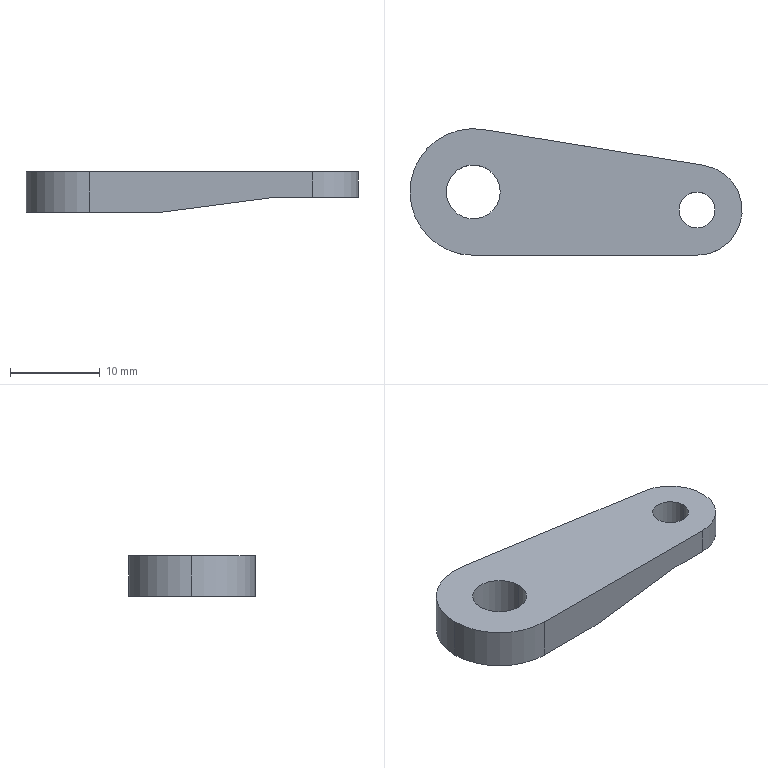Part | SolidWorks | features Extrusion 1, ICE 1 | 1 solid | 13 faces | box 36.997 x 14.091 x 4.508 mm | volume 1473 mm3 | cylinder 7 | plane 6 | commonest cylinder face diameters 4 x2 6 x2 14.091 x2 10.065 x1
STEP:
#1=CARTESIAN_POINT('',(-10.994,6.258,6.));
#2=VERTEX_POINT('',#1);
#3=CARTESIAN_POINT('',(-4.994,6.258,6.));
#4=VERTEX_POINT('',#3);
#5=CARTESIAN_POINT('',(-7.994,6.258,6.));
#6=DIRECTION('',(0.,0.,1.));
#7=DIRECTION('',(1.,0.,0.));
#8=AXIS2_PLACEMENT_3D('',#5,#6,#7);
#9=CIRCLE('',#8,3.);
#10=EDGE_CURVE('',#2,#4,#9,.T.);
#11=ORIENTED_EDGE('',*,*,#10,.T.);
#12=CARTESIAN_POINT('',(-4.994,6.258,1.492));
#13=VERTEX_POINT('',#12);
#14=CARTESIAN_POINT('',(-4.994,6.258,6.));
#15=DIRECTION('',(0.,0.,-1.));
#16=VECTOR('',#15,1000.);
#17=LINE('',#14,#16);
#18=EDGE_CURVE('',#4,#13,#17,.T.);
#19=ORIENTED_EDGE('',*,*,#18,.T.);
#20=CARTESIAN_POINT('',(-10.994,6.258,1.492));
#21=VERTEX_POINT('',#20);
#22=CARTESIAN_POINT('',(-7.994,6.258,1.492));
#23=DIRECTION('',(0.,0.,1.));
#24=DIRECTION('',(1.,0.,0.));
#25=AXIS2_PLACEMENT_3D('',#22,#23,#24);
#26=CIRCLE('',#25,3.);
#27=EDGE_CURVE('',#21,#13,#26,.T.);
#28=ORIENTED_EDGE('',*,*,#27,.F.);
#29=CARTESIAN_POINT('',(-10.994,6.258,6.));
#30=DIRECTION('',(0.,0.,-1.));
#31=VECTOR('',#30,1000.);
#32=LINE('',#29,#31);
#33=EDGE_CURVE('',#2,#21,#32,.T.);
#34=ORIENTED_EDGE('',*,*,#33,.F.);
#35=EDGE_LOOP('',(#11,#19,#28,#34));
#36=FACE_OUTER_BOUND('',#35,.T.);
#37=CARTESIAN_POINT('',(-7.994,6.258,6.));
#38=DIRECTION('',(0.,0.,-1.));
#39=DIRECTION('',(-1.,0.,0.));
#40=AXIS2_PLACEMENT_3D('',#37,#38,#39);
#41=CYLINDRICAL_SURFACE('',#40,3.);
#42=ADVANCED_FACE('',(#36),#41,.F.);
#43=CARTESIAN_POINT('',(14.925,4.245,6.));
#44=VERTEX_POINT('',#43);
#45=CARTESIAN_POINT('',(18.925,4.245,6.));
#46=VERTEX_POINT('',#45);
#47=CARTESIAN_POINT('',(16.925,4.245,6.));
#48=DIRECTION('',(0.,0.,1.));
#49=DIRECTION('',(1.,0.,0.));
#50=AXIS2_PLACEMENT_3D('',#47,#48,#49);
#51=CIRCLE('',#50,2.);
#52=EDGE_CURVE('',#44,#46,#51,.T.);
#53=ORIENTED_EDGE('',*,*,#52,.T.);
#54=CARTESIAN_POINT('',(18.925,4.245,3.142));
#55=VERTEX_POINT('',#54);
#56=CARTESIAN_POINT('',(18.925,4.245,6.));
#57=DIRECTION('',(0.,0.,-1.));
#58=VECTOR('',#57,1000.);
#59=LINE('',#56,#58);
#60=EDGE_CURVE('',#46,#55,#59,.T.);
#61=ORIENTED_EDGE('',*,*,#60,.T.);
#62=CARTESIAN_POINT('',(14.925,4.245,3.142));
#63=VERTEX_POINT('',#62);
#64=CARTESIAN_POINT('',(16.925,4.245,3.142));
#65=DIRECTION('',(0.,0.,1.));
#66=DIRECTION('',(1.,0.,0.));
#67=AXIS2_PLACEMENT_3D('',#64,#65,#66);
#68=CIRCLE('',#67,2.);
#69=EDGE_CURVE('',#63,#55,#68,.T.);
#70=ORIENTED_EDGE('',*,*,#69,.F.);
#71=CARTESIAN_POINT('',(14.925,4.245,6.));
#72=DIRECTION('',(0.,0.,-1.));
#73=VECTOR('',#72,1000.);
#74=LINE('',#71,#73);
#75=EDGE_CURVE('',#44,#63,#74,.T.);
#76=ORIENTED_EDGE('',*,*,#75,.F.);
#77=EDGE_LOOP('',(#53,#61,#70,#76));
#78=FACE_OUTER_BOUND('',#77,.T.);
#79=CARTESIAN_POINT('',(16.925,4.245,6.));
#80=DIRECTION('',(0.,0.,-1.));
#81=DIRECTION('',(-1.,0.,0.));
#82=AXIS2_PLACEMENT_3D('',#79,#80,#81);
#83=CYLINDRICAL_SURFACE('',#82,2.);
#84=ADVANCED_FACE('',(#78),#83,.F.);
#85=CARTESIAN_POINT('',(-15.039,6.258,6.));
#86=VERTEX_POINT('',#85);
#87=CARTESIAN_POINT('',(-7.994,-0.7875,6.));
#88=VERTEX_POINT('',#87);
#89=CARTESIAN_POINT('',(-7.994,6.258,6.));
#90=DIRECTION('',(0.,0.,1.));
#91=DIRECTION('',(1.,0.,0.));
#92=AXIS2_PLACEMENT_3D('',#89,#90,#91);
#93=CIRCLE('',#92,7.046);
#94=EDGE_CURVE('',#86,#88,#93,.T.);
#95=ORIENTED_EDGE('',*,*,#94,.F.);
#96=CARTESIAN_POINT('',(-15.039,6.258,1.492));
#97=VERTEX_POINT('',#96);
#98=CARTESIAN_POINT('',(-15.039,6.258,6.));
#99=DIRECTION('',(0.,0.,-1.));
#100=VECTOR('',#99,1000.);
#101=LINE('',#98,#100);
#102=EDGE_CURVE('',#86,#97,#101,.T.);
#103=ORIENTED_EDGE('',*,*,#102,.T.);
#104=CARTESIAN_POINT('',(-7.994,-0.7875,1.492));
#105=VERTEX_POINT('',#104);
#106=CARTESIAN_POINT('',(-7.994,6.258,1.492));
#107=DIRECTION('',(0.,0.,1.));
#108=DIRECTION('',(1.,0.,0.));
#109=AXIS2_PLACEMENT_3D('',#106,#107,#108);
#110=CIRCLE('',#109,7.046);
#111=EDGE_CURVE('',#97,#105,#110,.T.);
#112=ORIENTED_EDGE('',*,*,#111,.T.);
#113=CARTESIAN_POINT('',(-7.994,-0.7875,6.));
#114=DIRECTION('',(0.,0.,-1.));
#115=VECTOR('',#114,1000.);
#116=LINE('',#113,#115);
#117=EDGE_CURVE('',#88,#105,#116,.T.);
#118=ORIENTED_EDGE('',*,*,#117,.F.);
#119=EDGE_LOOP('',(#95,#103,#112,#118));
#120=FACE_OUTER_BOUND('',#119,.T.);
#121=CARTESIAN_POINT('',(-7.994,6.258,6.));
#122=DIRECTION('',(0.,0.,-1.));
#123=DIRECTION('',(-1.,0.,0.));
#124=AXIS2_PLACEMENT_3D('',#121,#122,#123);
#125=CYLINDRICAL_SURFACE('',#124,7.046);
#126=ADVANCED_FACE('',(#120),#125,.T.);
#127=ORIENTED_EDGE('',*,*,#52,.F.);
#128=CARTESIAN_POINT('',(16.925,4.245,6.));
#129=DIRECTION('',(0.,0.,1.));
#130=DIRECTION('',(1.,0.,0.));
#131=AXIS2_PLACEMENT_3D('',#128,#129,#130);
#132=CIRCLE('',#131,2.);
#133=EDGE_CURVE('',#46,#44,#132,.T.);
#134=ORIENTED_EDGE('',*,*,#133,.F.);
#135=EDGE_LOOP('',(#127,#134));
#136=FACE_BOUND('',#135,.T.);
#137=CARTESIAN_POINT('',(-6.863,13.213,6.));
#138=VERTEX_POINT('',#137);
#139=CARTESIAN_POINT('',(-7.994,6.258,6.));
#140=DIRECTION('',(0.,0.,1.));
#141=DIRECTION('',(1.,0.,0.));
#142=AXIS2_PLACEMENT_3D('',#139,#140,#141);
#143=CIRCLE('',#142,7.046);
#144=EDGE_CURVE('',#138,#86,#143,.T.);
#145=ORIENTED_EDGE('',*,*,#144,.T.);
#146=ORIENTED_EDGE('',*,*,#94,.T.);
#147=CARTESIAN_POINT('',(16.925,-0.7875,6.));
#148=VERTEX_POINT('',#147);
#149=CARTESIAN_POINT('',(-7.994,-0.7875,6.));
#150=DIRECTION('',(1.,0.,0.));
#151=VECTOR('',#150,1000.);
#152=LINE('',#149,#151);
#153=EDGE_CURVE('',#88,#148,#152,.T.);
#154=ORIENTED_EDGE('',*,*,#153,.T.);
#155=CARTESIAN_POINT('',(17.733,9.213,6.));
#156=VERTEX_POINT('',#155);
#157=CARTESIAN_POINT('',(16.925,4.245,6.));
#158=DIRECTION('',(0.,0.,1.));
#159=DIRECTION('',(-1.,0.,0.));
#160=AXIS2_PLACEMENT_3D('',#157,#158,#159);
#161=CIRCLE('',#160,5.033);
#162=EDGE_CURVE('',#148,#156,#161,.T.);
#163=ORIENTED_EDGE('',*,*,#162,.T.);
#164=CARTESIAN_POINT('',(-6.863,13.213,6.));
#165=DIRECTION('',(-0.987,0.1605,0.));
#166=VECTOR('',#165,1000.);
#167=LINE('',#164,#166);
#168=EDGE_CURVE('',#156,#138,#167,.T.);
#169=ORIENTED_EDGE('',*,*,#168,.T.);
#170=EDGE_LOOP('',(#145,#146,#154,#163,#169));
#171=FACE_OUTER_BOUND('',#170,.T.);
#172=ORIENTED_EDGE('',*,*,#10,.F.);
#173=CARTESIAN_POINT('',(-7.994,6.258,6.));
#174=DIRECTION('',(0.,0.,1.));
#175=DIRECTION('',(1.,0.,0.));
#176=AXIS2_PLACEMENT_3D('',#173,#174,#175);
#177=CIRCLE('',#176,3.);
#178=EDGE_CURVE('',#4,#2,#177,.T.);
#179=ORIENTED_EDGE('',*,*,#178,.F.);
#180=EDGE_LOOP('',(#172,#179));
#181=FACE_BOUND('',#180,.T.);
#182=CARTESIAN_POINT('',(-7.994,6.258,6.));
#183=DIRECTION('',(0.,0.,1.));
#184=DIRECTION('',(1.,0.,0.));
#185=AXIS2_PLACEMENT_3D('',#182,#183,#184);
#186=PLANE('',#185);
#187=ADVANCED_FACE('',(#136,#171,#181),#186,.T.);
#188=ORIENTED_EDGE('',*,*,#102,.F.);
#189=ORIENTED_EDGE('',*,*,#144,.F.);
#190=CARTESIAN_POINT('',(-6.863,13.213,1.492));
#191=VERTEX_POINT('',#190);
#192=CARTESIAN_POINT('',(-6.863,13.213,6.));
#193=DIRECTION('',(0.,0.,-1.));
#194=VECTOR('',#193,1000.);
#195=LINE('',#192,#194);
#196=EDGE_CURVE('',#138,#191,#195,.T.);
#197=ORIENTED_EDGE('',*,*,#196,.T.);
#198=CARTESIAN_POINT('',(-7.994,6.258,1.492));
#199=DIRECTION('',(0.,0.,1.));
#200=DIRECTION('',(1.,0.,0.));
#201=AXIS2_PLACEMENT_3D('',#198,#199,#200);
#202=CIRCLE('',#201,7.046);
#203=EDGE_CURVE('',#191,#97,#202,.T.);
#204=ORIENTED_EDGE('',*,*,#203,.T.);
#205=EDGE_LOOP('',(#188,#189,#197,#204));
#206=FACE_OUTER_BOUND('',#205,.T.);
#207=CARTESIAN_POINT('',(-7.994,6.258,6.));
#208=DIRECTION('',(0.,0.,-1.));
#209=DIRECTION('',(-1.,0.,0.));
#210=AXIS2_PLACEMENT_3D('',#207,#208,#209);
#211=CYLINDRICAL_SURFACE('',#210,7.046);
#212=ADVANCED_FACE('',(#206),#211,.T.);
#213=CARTESIAN_POINT('',(0.,-0.7875,1.492));
#214=VERTEX_POINT('',#213);
#215=CARTESIAN_POINT('',(12.581,-0.7875,3.142));
#216=VERTEX_POINT('',#215);
#217=CARTESIAN_POINT('',(12.581,-0.7875,3.142));
#218=DIRECTION('',(0.9915,0.,0.13));
#219=VECTOR('',#218,1000.);
#220=LINE('',#217,#219);
#221=EDGE_CURVE('',#214,#216,#220,.T.);
#222=ORIENTED_EDGE('',*,*,#221,.T.);
#223=CARTESIAN_POINT('',(16.925,-0.7875,3.142));
#224=VERTEX_POINT('',#223);
#225=CARTESIAN_POINT('',(29.387,-0.7875,3.142));
#226=DIRECTION('',(1.,0.,0.));
#227=VECTOR('',#226,1000.);
#228=LINE('',#225,#227);
#229=EDGE_CURVE('',#216,#224,#228,.T.);
#230=ORIENTED_EDGE('',*,*,#229,.T.);
#231=CARTESIAN_POINT('',(16.925,-0.7875,6.));
#232=DIRECTION('',(0.,0.,-1.));
#233=VECTOR('',#232,1000.);
#234=LINE('',#231,#233);
#235=EDGE_CURVE('',#148,#224,#234,.T.);
#236=ORIENTED_EDGE('',*,*,#235,.F.);
#237=ORIENTED_EDGE('',*,*,#153,.F.);
#238=ORIENTED_EDGE('',*,*,#117,.T.);
#239=CARTESIAN_POINT('',(0.,-0.7875,1.492));
#240=DIRECTION('',(1.,0.,0.));
#241=VECTOR('',#240,1000.);
#242=LINE('',#239,#241);
#243=EDGE_CURVE('',#105,#214,#242,.T.);
#244=ORIENTED_EDGE('',*,*,#243,.T.);
#245=EDGE_LOOP('',(#222,#230,#236,#237,#238,#244));
#246=FACE_OUTER_BOUND('',#245,.T.);
#247=CARTESIAN_POINT('',(-7.994,-0.7875,6.));
#248=DIRECTION('',(0.,1.,0.));
#249=DIRECTION('',(0.,0.,1.));
#250=AXIS2_PLACEMENT_3D('',#247,#248,#249);
#251=PLANE('',#250);
#252=ADVANCED_FACE('',(#246),#251,.F.);
#253=ORIENTED_EDGE('',*,*,#235,.T.);
#254=CARTESIAN_POINT('',(17.733,9.213,3.142));
#255=VERTEX_POINT('',#254);
#256=CARTESIAN_POINT('',(16.925,4.245,3.142));
#257=DIRECTION('',(0.,0.,1.));
#258=DIRECTION('',(1.,0.,0.));
#259=AXIS2_PLACEMENT_3D('',#256,#257,#258);
#260=CIRCLE('',#259,5.033);
#261=EDGE_CURVE('',#224,#255,#260,.T.);
#262=ORIENTED_EDGE('',*,*,#261,.T.);
#263=CARTESIAN_POINT('',(17.733,9.213,6.));
#264=DIRECTION('',(0.,0.,-1.));
#265=VECTOR('',#264,1000.);
#266=LINE('',#263,#265);
#267=EDGE_CURVE('',#156,#255,#266,.T.);
#268=ORIENTED_EDGE('',*,*,#267,.F.);
#269=ORIENTED_EDGE('',*,*,#162,.F.);
#270=EDGE_LOOP('',(#253,#262,#268,#269));
#271=FACE_OUTER_BOUND('',#270,.T.);
#272=CARTESIAN_POINT('',(16.925,4.245,6.));
#273=DIRECTION('',(0.,0.,-1.));
#274=DIRECTION('',(-1.,0.,0.));
#275=AXIS2_PLACEMENT_3D('',#272,#273,#274);
#276=CYLINDRICAL_SURFACE('',#275,5.033);
#277=ADVANCED_FACE('',(#271),#276,.T.);
#278=ORIENTED_EDGE('',*,*,#267,.T.);
#279=CARTESIAN_POINT('',(12.581,10.05,3.142));
#280=VERTEX_POINT('',#279);
#281=CARTESIAN_POINT('',(-6.863,13.213,3.142));
#282=DIRECTION('',(-0.987,0.1605,0.));
#283=VECTOR('',#282,1000.);
#284=LINE('',#281,#283);
#285=EDGE_CURVE('',#255,#280,#284,.T.);
#286=ORIENTED_EDGE('',*,*,#285,.T.);
#287=CARTESIAN_POINT('',(0.,12.096,1.492));
#288=VERTEX_POINT('',#287);
#289=CARTESIAN_POINT('',(-6.183,13.102,0.6809));
#290=DIRECTION('',(-0.9789,0.1592,-0.1284));
#291=VECTOR('',#290,1000.);
#292=LINE('',#289,#291);
#293=EDGE_CURVE('',#280,#288,#292,.T.);
#294=ORIENTED_EDGE('',*,*,#293,.T.);
#295=CARTESIAN_POINT('',(-6.863,13.213,1.492));
#296=DIRECTION('',(-0.987,0.1605,0.));
#297=VECTOR('',#296,1000.);
#298=LINE('',#295,#297);
#299=EDGE_CURVE('',#288,#191,#298,.T.);
#300=ORIENTED_EDGE('',*,*,#299,.T.);
#301=ORIENTED_EDGE('',*,*,#196,.F.);
#302=ORIENTED_EDGE('',*,*,#168,.F.);
#303=EDGE_LOOP('',(#278,#286,#294,#300,#301,#302));
#304=FACE_OUTER_BOUND('',#303,.T.);
#305=CARTESIAN_POINT('',(-6.863,13.213,6.));
#306=DIRECTION('',(-0.1605,-0.987,0.));
#307=DIRECTION('',(0.987,-0.1605,0.));
#308=AXIS2_PLACEMENT_3D('',#305,#306,#307);
#309=PLANE('',#308);
#310=ADVANCED_FACE('',(#304),#309,.F.);
#311=ORIENTED_EDGE('',*,*,#60,.F.);
#312=ORIENTED_EDGE('',*,*,#133,.T.);
#313=ORIENTED_EDGE('',*,*,#75,.T.);
#314=CARTESIAN_POINT('',(16.925,4.245,3.142));
#315=DIRECTION('',(0.,0.,1.));
#316=DIRECTION('',(1.,0.,0.));
#317=AXIS2_PLACEMENT_3D('',#314,#315,#316);
#318=CIRCLE('',#317,2.);
#319=EDGE_CURVE('',#55,#63,#318,.T.);
#320=ORIENTED_EDGE('',*,*,#319,.F.);
#321=EDGE_LOOP('',(#311,#312,#313,#320));
#322=FACE_OUTER_BOUND('',#321,.T.);
#323=CARTESIAN_POINT('',(16.925,4.245,6.));
#324=DIRECTION('',(0.,0.,-1.));
#325=DIRECTION('',(-1.,0.,0.));
#326=AXIS2_PLACEMENT_3D('',#323,#324,#325);
#327=CYLINDRICAL_SURFACE('',#326,2.);
#328=ADVANCED_FACE('',(#322),#327,.F.);
#329=ORIENTED_EDGE('',*,*,#18,.F.);
#330=ORIENTED_EDGE('',*,*,#178,.T.);
#331=ORIENTED_EDGE('',*,*,#33,.T.);
#332=CARTESIAN_POINT('',(-7.994,6.258,1.492));
#333=DIRECTION('',(0.,0.,1.));
#334=DIRECTION('',(1.,0.,0.));
#335=AXIS2_PLACEMENT_3D('',#332,#333,#334);
#336=CIRCLE('',#335,3.);
#337=EDGE_CURVE('',#13,#21,#336,.T.);
#338=ORIENTED_EDGE('',*,*,#337,.F.);
#339=EDGE_LOOP('',(#329,#330,#331,#338));
#340=FACE_OUTER_BOUND('',#339,.T.);
#341=CARTESIAN_POINT('',(-7.994,6.258,6.));
#342=DIRECTION('',(0.,0.,-1.));
#343=DIRECTION('',(-1.,0.,0.));
#344=AXIS2_PLACEMENT_3D('',#341,#342,#343);
#345=CYLINDRICAL_SURFACE('',#344,3.);
#346=ADVANCED_FACE('',(#340),#345,.F.);
#347=CARTESIAN_POINT('',(12.581,-0.7875,3.142));
#348=DIRECTION('',(0.,1.,0.));
#349=VECTOR('',#348,1000.);
#350=LINE('',#347,#349);
#351=EDGE_CURVE('',#216,#280,#350,.T.);
#352=ORIENTED_EDGE('',*,*,#351,.F.);
#353=ORIENTED_EDGE('',*,*,#221,.F.);
#354=CARTESIAN_POINT('',(0.,-0.7875,1.492));
#355=DIRECTION('',(0.,1.,0.));
#356=VECTOR('',#355,1000.);
#357=LINE('',#354,#356);
#358=EDGE_CURVE('',#214,#288,#357,.T.);
#359=ORIENTED_EDGE('',*,*,#358,.T.);
#360=ORIENTED_EDGE('',*,*,#293,.F.);
#361=EDGE_LOOP('',(#352,#353,#359,#360));
#362=FACE_OUTER_BOUND('',#361,.T.);
#363=CARTESIAN_POINT('',(12.581,-0.7875,3.142));
#364=DIRECTION('',(-0.13,0.,0.9915));
#365=DIRECTION('',(0.9915,0.,0.13));
#366=AXIS2_PLACEMENT_3D('',#363,#364,#365);
#367=PLANE('',#366);
#368=ADVANCED_FACE('',(#362),#367,.F.);
#369=ORIENTED_EDGE('',*,*,#69,.T.);
#370=ORIENTED_EDGE('',*,*,#319,.T.);
#371=EDGE_LOOP('',(#369,#370));
#372=FACE_BOUND('',#371,.T.);
#373=ORIENTED_EDGE('',*,*,#229,.F.);
#374=ORIENTED_EDGE('',*,*,#351,.T.);
#375=ORIENTED_EDGE('',*,*,#285,.F.);
#376=ORIENTED_EDGE('',*,*,#261,.F.);
#377=EDGE_LOOP('',(#373,#374,#375,#376));
#378=FACE_OUTER_BOUND('',#377,.T.);
#379=CARTESIAN_POINT('',(29.387,-0.7875,3.142));
#380=DIRECTION('',(0.,0.,1.));
#381=DIRECTION('',(1.,0.,0.));
#382=AXIS2_PLACEMENT_3D('',#379,#380,#381);
#383=PLANE('',#382);
#384=ADVANCED_FACE('',(#372,#378),#383,.F.);
#385=ORIENTED_EDGE('',*,*,#27,.T.);
#386=ORIENTED_EDGE('',*,*,#337,.T.);
#387=EDGE_LOOP('',(#385,#386));
#388=FACE_BOUND('',#387,.T.);
#389=ORIENTED_EDGE('',*,*,#203,.F.);
#390=ORIENTED_EDGE('',*,*,#299,.F.);
#391=ORIENTED_EDGE('',*,*,#358,.F.);
#392=ORIENTED_EDGE('',*,*,#243,.F.);
#393=ORIENTED_EDGE('',*,*,#111,.F.);
#394=EDGE_LOOP('',(#389,#390,#391,#392,#393));
#395=FACE_OUTER_BOUND('',#394,.T.);
#396=CARTESIAN_POINT('',(0.,-0.7875,1.492));
#397=DIRECTION('',(0.,0.,1.));
#398=DIRECTION('',(1.,0.,0.));
#399=AXIS2_PLACEMENT_3D('',#396,#397,#398);
#400=PLANE('',#399);
#401=ADVANCED_FACE('',(#388,#395),#400,.F.);
#402=CLOSED_SHELL('',(#42,#84,#126,#187,#212,#252,#277,#310,#328,#346,#368,#384,#401));
#403=MANIFOLD_SOLID_BREP('',#402);
#404=CARTESIAN_POINT('',(0.,0.,0.));
#405=DIRECTION('',(0.,0.,1.));
#406=DIRECTION('',(1.,0.,0.));
#407=AXIS2_PLACEMENT_3D('',#404,#405,#406);
#408=(LENGTH_UNIT()NAMED_UNIT(*)SI_UNIT(.MILLI.,.METRE.));
#409=UNCERTAINTY_MEASURE_WITH_UNIT(LENGTH_MEASURE(0.00001),#408,'','');
#410=(NAMED_UNIT(*)PLANE_ANGLE_UNIT()SI_UNIT($,.RADIAN.));
#411=(NAMED_UNIT(*)SI_UNIT($,.STERADIAN.)SOLID_ANGLE_UNIT());
#412=(GEOMETRIC_REPRESENTATION_CONTEXT(3)GLOBAL_UNCERTAINTY_ASSIGNED_CONTEXT((#409))GLOBAL_UNIT_ASSIGNED_CONTEXT((#408,#410,#411))REPRESENTATION_CONTEXT('',''));
#413=ADVANCED_BREP_SHAPE_REPRESENTATION('',(#403,#407),#412);